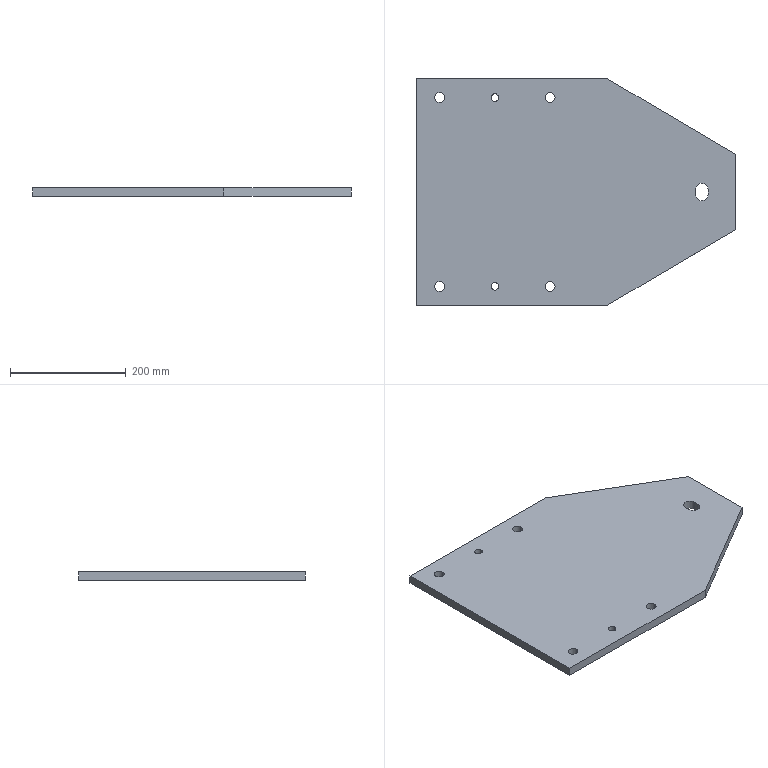Part | SolidWorks | features Extrusion 1, ICE 1 | 1 solid | 24 faces | box 550 x 390 x 15 mm | volume 2762557 mm3 | cylinder 14 | plane 10 | commonest cylinder face diameters 17 x8 13 x4 22 x2
STEP:
#1=CARTESIAN_POINT('',(-146.5,163.,0.));
#2=VERTEX_POINT('',#1);
#3=CARTESIAN_POINT('',(-133.5,163.,0.));
#4=VERTEX_POINT('',#3);
#5=CARTESIAN_POINT('',(-140.,163.,0.));
#6=DIRECTION('',(0.,0.,1.));
#7=DIRECTION('',(1.,0.,0.));
#8=AXIS2_PLACEMENT_3D('',#5,#6,#7);
#9=CIRCLE('',#8,6.5);
#10=EDGE_CURVE('',#2,#4,#9,.T.);
#11=ORIENTED_EDGE('',*,*,#10,.F.);
#12=CARTESIAN_POINT('',(-146.5,163.,15.));
#13=VERTEX_POINT('',#12);
#14=CARTESIAN_POINT('',(-146.5,163.,0.));
#15=DIRECTION('',(0.,0.,1.));
#16=VECTOR('',#15,1000.);
#17=LINE('',#14,#16);
#18=EDGE_CURVE('',#2,#13,#17,.T.);
#19=ORIENTED_EDGE('',*,*,#18,.T.);
#20=CARTESIAN_POINT('',(-133.5,163.,15.));
#21=VERTEX_POINT('',#20);
#22=CARTESIAN_POINT('',(-140.,163.,15.));
#23=DIRECTION('',(0.,0.,1.));
#24=DIRECTION('',(1.,0.,0.));
#25=AXIS2_PLACEMENT_3D('',#22,#23,#24);
#26=CIRCLE('',#25,6.5);
#27=EDGE_CURVE('',#13,#21,#26,.T.);
#28=ORIENTED_EDGE('',*,*,#27,.T.);
#29=CARTESIAN_POINT('',(-133.5,163.,0.));
#30=DIRECTION('',(0.,0.,1.));
#31=VECTOR('',#30,1000.);
#32=LINE('',#29,#31);
#33=EDGE_CURVE('',#4,#21,#32,.T.);
#34=ORIENTED_EDGE('',*,*,#33,.F.);
#35=EDGE_LOOP('',(#11,#19,#28,#34));
#36=FACE_OUTER_BOUND('',#35,.T.);
#37=CARTESIAN_POINT('',(-140.,163.,0.));
#38=DIRECTION('',(0.,0.,1.));
#39=DIRECTION('',(1.,0.,0.));
#40=AXIS2_PLACEMENT_3D('',#37,#38,#39);
#41=CYLINDRICAL_SURFACE('',#40,6.5);
#42=ADVANCED_FACE('',(#36),#41,.F.);
#43=CARTESIAN_POINT('',(-53.2,-163.,0.));
#44=VERTEX_POINT('',#43);
#45=CARTESIAN_POINT('',(-36.2,-163.,0.));
#46=VERTEX_POINT('',#45);
#47=CARTESIAN_POINT('',(-44.7,-163.,0.));
#48=DIRECTION('',(0.,0.,1.));
#49=DIRECTION('',(1.,0.,0.));
#50=AXIS2_PLACEMENT_3D('',#47,#48,#49);
#51=CIRCLE('',#50,8.5);
#52=EDGE_CURVE('',#44,#46,#51,.T.);
#53=ORIENTED_EDGE('',*,*,#52,.F.);
#54=CARTESIAN_POINT('',(-53.2,-163.,15.));
#55=VERTEX_POINT('',#54);
#56=CARTESIAN_POINT('',(-53.2,-163.,0.));
#57=DIRECTION('',(0.,0.,1.));
#58=VECTOR('',#57,1000.);
#59=LINE('',#56,#58);
#60=EDGE_CURVE('',#44,#55,#59,.T.);
#61=ORIENTED_EDGE('',*,*,#60,.T.);
#62=CARTESIAN_POINT('',(-36.2,-163.,15.));
#63=VERTEX_POINT('',#62);
#64=CARTESIAN_POINT('',(-44.7,-163.,15.));
#65=DIRECTION('',(0.,0.,1.));
#66=DIRECTION('',(1.,0.,0.));
#67=AXIS2_PLACEMENT_3D('',#64,#65,#66);
#68=CIRCLE('',#67,8.5);
#69=EDGE_CURVE('',#55,#63,#68,.T.);
#70=ORIENTED_EDGE('',*,*,#69,.T.);
#71=CARTESIAN_POINT('',(-36.2,-163.,0.));
#72=DIRECTION('',(0.,0.,1.));
#73=VECTOR('',#72,1000.);
#74=LINE('',#71,#73);
#75=EDGE_CURVE('',#46,#63,#74,.T.);
#76=ORIENTED_EDGE('',*,*,#75,.F.);
#77=EDGE_LOOP('',(#53,#61,#70,#76));
#78=FACE_OUTER_BOUND('',#77,.T.);
#79=CARTESIAN_POINT('',(-44.7,-163.,0.));
#80=DIRECTION('',(0.,0.,1.));
#81=DIRECTION('',(1.,0.,0.));
#82=AXIS2_PLACEMENT_3D('',#79,#80,#81);
#83=CYLINDRICAL_SURFACE('',#82,8.5);
#84=ADVANCED_FACE('',(#78),#83,.F.);
#85=CARTESIAN_POINT('',(-146.5,-163.,0.));
#86=VERTEX_POINT('',#85);
#87=CARTESIAN_POINT('',(-133.5,-163.,0.));
#88=VERTEX_POINT('',#87);
#89=CARTESIAN_POINT('',(-140.,-163.,0.));
#90=DIRECTION('',(0.,0.,1.));
#91=DIRECTION('',(1.,0.,0.));
#92=AXIS2_PLACEMENT_3D('',#89,#90,#91);
#93=CIRCLE('',#92,6.5);
#94=EDGE_CURVE('',#86,#88,#93,.T.);
#95=ORIENTED_EDGE('',*,*,#94,.F.);
#96=CARTESIAN_POINT('',(-146.5,-163.,15.));
#97=VERTEX_POINT('',#96);
#98=CARTESIAN_POINT('',(-146.5,-163.,0.));
#99=DIRECTION('',(0.,0.,1.));
#100=VECTOR('',#99,1000.);
#101=LINE('',#98,#100);
#102=EDGE_CURVE('',#86,#97,#101,.T.);
#103=ORIENTED_EDGE('',*,*,#102,.T.);
#104=CARTESIAN_POINT('',(-133.5,-163.,15.));
#105=VERTEX_POINT('',#104);
#106=CARTESIAN_POINT('',(-140.,-163.,15.));
#107=DIRECTION('',(0.,0.,1.));
#108=DIRECTION('',(1.,0.,0.));
#109=AXIS2_PLACEMENT_3D('',#106,#107,#108);
#110=CIRCLE('',#109,6.5);
#111=EDGE_CURVE('',#97,#105,#110,.T.);
#112=ORIENTED_EDGE('',*,*,#111,.T.);
#113=CARTESIAN_POINT('',(-133.5,-163.,0.));
#114=DIRECTION('',(0.,0.,1.));
#115=VECTOR('',#114,1000.);
#116=LINE('',#113,#115);
#117=EDGE_CURVE('',#88,#105,#116,.T.);
#118=ORIENTED_EDGE('',*,*,#117,.F.);
#119=EDGE_LOOP('',(#95,#103,#112,#118));
#120=FACE_OUTER_BOUND('',#119,.T.);
#121=CARTESIAN_POINT('',(-140.,-163.,0.));
#122=DIRECTION('',(0.,0.,1.));
#123=DIRECTION('',(1.,0.,0.));
#124=AXIS2_PLACEMENT_3D('',#121,#122,#123);
#125=CYLINDRICAL_SURFACE('',#124,6.5);
#126=ADVANCED_FACE('',(#120),#125,.F.);
#127=CARTESIAN_POINT('',(-243.7,-163.,0.));
#128=VERTEX_POINT('',#127);
#129=CARTESIAN_POINT('',(-226.7,-163.,0.));
#130=VERTEX_POINT('',#129);
#131=CARTESIAN_POINT('',(-235.2,-163.,0.));
#132=DIRECTION('',(0.,0.,1.));
#133=DIRECTION('',(1.,0.,0.));
#134=AXIS2_PLACEMENT_3D('',#131,#132,#133);
#135=CIRCLE('',#134,8.5);
#136=EDGE_CURVE('',#128,#130,#135,.T.);
#137=ORIENTED_EDGE('',*,*,#136,.F.);
#138=CARTESIAN_POINT('',(-243.7,-163.,15.));
#139=VERTEX_POINT('',#138);
#140=CARTESIAN_POINT('',(-243.7,-163.,0.));
#141=DIRECTION('',(0.,0.,1.));
#142=VECTOR('',#141,1000.);
#143=LINE('',#140,#142);
#144=EDGE_CURVE('',#128,#139,#143,.T.);
#145=ORIENTED_EDGE('',*,*,#144,.T.);
#146=CARTESIAN_POINT('',(-226.7,-163.,15.));
#147=VERTEX_POINT('',#146);
#148=CARTESIAN_POINT('',(-235.2,-163.,15.));
#149=DIRECTION('',(0.,0.,1.));
#150=DIRECTION('',(1.,0.,0.));
#151=AXIS2_PLACEMENT_3D('',#148,#149,#150);
#152=CIRCLE('',#151,8.5);
#153=EDGE_CURVE('',#139,#147,#152,.T.);
#154=ORIENTED_EDGE('',*,*,#153,.T.);
#155=CARTESIAN_POINT('',(-226.7,-163.,0.));
#156=DIRECTION('',(0.,0.,1.));
#157=VECTOR('',#156,1000.);
#158=LINE('',#155,#157);
#159=EDGE_CURVE('',#130,#147,#158,.T.);
#160=ORIENTED_EDGE('',*,*,#159,.F.);
#161=EDGE_LOOP('',(#137,#145,#154,#160));
#162=FACE_OUTER_BOUND('',#161,.T.);
#163=CARTESIAN_POINT('',(-235.2,-163.,0.));
#164=DIRECTION('',(0.,0.,1.));
#165=DIRECTION('',(1.,0.,0.));
#166=AXIS2_PLACEMENT_3D('',#163,#164,#165);
#167=CYLINDRICAL_SURFACE('',#166,8.5);
#168=ADVANCED_FACE('',(#162),#167,.F.);
#169=CARTESIAN_POINT('',(-53.2,163.,0.));
#170=VERTEX_POINT('',#169);
#171=CARTESIAN_POINT('',(-36.2,163.,0.));
#172=VERTEX_POINT('',#171);
#173=CARTESIAN_POINT('',(-44.7,163.,0.));
#174=DIRECTION('',(0.,0.,1.));
#175=DIRECTION('',(1.,0.,0.));
#176=AXIS2_PLACEMENT_3D('',#173,#174,#175);
#177=CIRCLE('',#176,8.5);
#178=EDGE_CURVE('',#170,#172,#177,.T.);
#179=ORIENTED_EDGE('',*,*,#178,.F.);
#180=CARTESIAN_POINT('',(-53.2,163.,15.));
#181=VERTEX_POINT('',#180);
#182=CARTESIAN_POINT('',(-53.2,163.,0.));
#183=DIRECTION('',(0.,0.,1.));
#184=VECTOR('',#183,1000.);
#185=LINE('',#182,#184);
#186=EDGE_CURVE('',#170,#181,#185,.T.);
#187=ORIENTED_EDGE('',*,*,#186,.T.);
#188=CARTESIAN_POINT('',(-36.2,163.,15.));
#189=VERTEX_POINT('',#188);
#190=CARTESIAN_POINT('',(-44.7,163.,15.));
#191=DIRECTION('',(0.,0.,1.));
#192=DIRECTION('',(1.,0.,0.));
#193=AXIS2_PLACEMENT_3D('',#190,#191,#192);
#194=CIRCLE('',#193,8.5);
#195=EDGE_CURVE('',#181,#189,#194,.T.);
#196=ORIENTED_EDGE('',*,*,#195,.T.);
#197=CARTESIAN_POINT('',(-36.2,163.,0.));
#198=DIRECTION('',(0.,0.,1.));
#199=VECTOR('',#198,1000.);
#200=LINE('',#197,#199);
#201=EDGE_CURVE('',#172,#189,#200,.T.);
#202=ORIENTED_EDGE('',*,*,#201,.F.);
#203=EDGE_LOOP('',(#179,#187,#196,#202));
#204=FACE_OUTER_BOUND('',#203,.T.);
#205=CARTESIAN_POINT('',(-44.7,163.,0.));
#206=DIRECTION('',(0.,0.,1.));
#207=DIRECTION('',(1.,0.,0.));
#208=AXIS2_PLACEMENT_3D('',#205,#206,#207);
#209=CYLINDRICAL_SURFACE('',#208,8.5);
#210=ADVANCED_FACE('',(#204),#209,.F.);
#211=CARTESIAN_POINT('',(-243.7,163.,0.));
#212=VERTEX_POINT('',#211);
#213=CARTESIAN_POINT('',(-226.7,163.,0.));
#214=VERTEX_POINT('',#213);
#215=CARTESIAN_POINT('',(-235.2,163.,0.));
#216=DIRECTION('',(0.,0.,1.));
#217=DIRECTION('',(1.,0.,0.));
#218=AXIS2_PLACEMENT_3D('',#215,#216,#217);
#219=CIRCLE('',#218,8.5);
#220=EDGE_CURVE('',#212,#214,#219,.T.);
#221=ORIENTED_EDGE('',*,*,#220,.F.);
#222=CARTESIAN_POINT('',(-243.7,163.,15.));
#223=VERTEX_POINT('',#222);
#224=CARTESIAN_POINT('',(-243.7,163.,0.));
#225=DIRECTION('',(0.,0.,1.));
#226=VECTOR('',#225,1000.);
#227=LINE('',#224,#226);
#228=EDGE_CURVE('',#212,#223,#227,.T.);
#229=ORIENTED_EDGE('',*,*,#228,.T.);
#230=CARTESIAN_POINT('',(-226.7,163.,15.));
#231=VERTEX_POINT('',#230);
#232=CARTESIAN_POINT('',(-235.2,163.,15.));
#233=DIRECTION('',(0.,0.,1.));
#234=DIRECTION('',(1.,0.,0.));
#235=AXIS2_PLACEMENT_3D('',#232,#233,#234);
#236=CIRCLE('',#235,8.5);
#237=EDGE_CURVE('',#223,#231,#236,.T.);
#238=ORIENTED_EDGE('',*,*,#237,.T.);
#239=CARTESIAN_POINT('',(-226.7,163.,0.));
#240=DIRECTION('',(0.,0.,1.));
#241=VECTOR('',#240,1000.);
#242=LINE('',#239,#241);
#243=EDGE_CURVE('',#214,#231,#242,.T.);
#244=ORIENTED_EDGE('',*,*,#243,.F.);
#245=EDGE_LOOP('',(#221,#229,#238,#244));
#246=FACE_OUTER_BOUND('',#245,.T.);
#247=CARTESIAN_POINT('',(-235.2,163.,0.));
#248=DIRECTION('',(0.,0.,1.));
#249=DIRECTION('',(1.,0.,0.));
#250=AXIS2_PLACEMENT_3D('',#247,#248,#249);
#251=CYLINDRICAL_SURFACE('',#250,8.5);
#252=ADVANCED_FACE('',(#246),#251,.F.);
#253=CARTESIAN_POINT('',(-275.,195.,0.));
#254=VERTEX_POINT('',#253);
#255=CARTESIAN_POINT('',(-275.,-195.,0.));
#256=VERTEX_POINT('',#255);
#257=CARTESIAN_POINT('',(-275.,195.,0.));
#258=DIRECTION('',(0.,-1.,0.));
#259=VECTOR('',#258,1000.);
#260=LINE('',#257,#259);
#261=EDGE_CURVE('',#254,#256,#260,.T.);
#262=ORIENTED_EDGE('',*,*,#261,.T.);
#263=CARTESIAN_POINT('',(-275.,-195.,15.));
#264=VERTEX_POINT('',#263);
#265=CARTESIAN_POINT('',(-275.,-195.,15.));
#266=DIRECTION('',(0.,0.,-1.));
#267=VECTOR('',#266,1000.);
#268=LINE('',#265,#267);
#269=EDGE_CURVE('',#264,#256,#268,.T.);
#270=ORIENTED_EDGE('',*,*,#269,.F.);
#271=CARTESIAN_POINT('',(-275.,195.,15.));
#272=VERTEX_POINT('',#271);
#273=CARTESIAN_POINT('',(-275.,195.,15.));
#274=DIRECTION('',(0.,-1.,0.));
#275=VECTOR('',#274,1000.);
#276=LINE('',#273,#275);
#277=EDGE_CURVE('',#272,#264,#276,.T.);
#278=ORIENTED_EDGE('',*,*,#277,.F.);
#279=CARTESIAN_POINT('',(-275.,195.,15.));
#280=DIRECTION('',(0.,0.,-1.));
#281=VECTOR('',#280,1000.);
#282=LINE('',#279,#281);
#283=EDGE_CURVE('',#272,#254,#282,.T.);
#284=ORIENTED_EDGE('',*,*,#283,.T.);
#285=EDGE_LOOP('',(#262,#270,#278,#284));
#286=FACE_OUTER_BOUND('',#285,.T.);
#287=CARTESIAN_POINT('',(-275.,195.,15.));
#288=DIRECTION('',(1.,0.,0.));
#289=DIRECTION('',(0.,1.,0.));
#290=AXIS2_PLACEMENT_3D('',#287,#288,#289);
#291=PLANE('',#290);
#292=ADVANCED_FACE('',(#286),#291,.F.);
#293=CARTESIAN_POINT('',(55.,-195.,0.));
#294=VERTEX_POINT('',#293);
#295=CARTESIAN_POINT('',(275.,-195.,0.));
#296=DIRECTION('',(1.,0.,0.));
#297=VECTOR('',#296,1000.);
#298=LINE('',#295,#297);
#299=EDGE_CURVE('',#256,#294,#298,.T.);
#300=ORIENTED_EDGE('',*,*,#299,.T.);
#301=CARTESIAN_POINT('',(55.,-195.,15.));
#302=VERTEX_POINT('',#301);
#303=CARTESIAN_POINT('',(55.,-195.,0.));
#304=DIRECTION('',(0.,0.,1.));
#305=VECTOR('',#304,1000.);
#306=LINE('',#303,#305);
#307=EDGE_CURVE('',#294,#302,#306,.T.);
#308=ORIENTED_EDGE('',*,*,#307,.T.);
#309=CARTESIAN_POINT('',(275.,-195.,15.));
#310=DIRECTION('',(1.,0.,0.));
#311=VECTOR('',#310,1000.);
#312=LINE('',#309,#311);
#313=EDGE_CURVE('',#264,#302,#312,.T.);
#314=ORIENTED_EDGE('',*,*,#313,.F.);
#315=ORIENTED_EDGE('',*,*,#269,.T.);
#316=EDGE_LOOP('',(#300,#308,#314,#315));
#317=FACE_OUTER_BOUND('',#316,.T.);
#318=CARTESIAN_POINT('',(275.,-195.,15.));
#319=DIRECTION('',(0.,1.,0.));
#320=DIRECTION('',(-1.,0.,0.));
#321=AXIS2_PLACEMENT_3D('',#318,#319,#320);
#322=PLANE('',#321);
#323=ADVANCED_FACE('',(#317),#322,.F.);
#324=CARTESIAN_POINT('',(275.,-65.,0.));
#325=VERTEX_POINT('',#324);
#326=CARTESIAN_POINT('',(275.,65.,0.));
#327=VERTEX_POINT('',#326);
#328=CARTESIAN_POINT('',(275.,195.,0.));
#329=DIRECTION('',(0.,1.,0.));
#330=VECTOR('',#329,1000.);
#331=LINE('',#328,#330);
#332=EDGE_CURVE('',#325,#327,#331,.T.);
#333=ORIENTED_EDGE('',*,*,#332,.T.);
#334=CARTESIAN_POINT('',(275.,65.,15.));
#335=VERTEX_POINT('',#334);
#336=CARTESIAN_POINT('',(275.,65.,0.));
#337=DIRECTION('',(0.,0.,1.));
#338=VECTOR('',#337,1000.);
#339=LINE('',#336,#338);
#340=EDGE_CURVE('',#327,#335,#339,.T.);
#341=ORIENTED_EDGE('',*,*,#340,.T.);
#342=CARTESIAN_POINT('',(275.,-65.,15.));
#343=VERTEX_POINT('',#342);
#344=CARTESIAN_POINT('',(275.,195.,15.));
#345=DIRECTION('',(0.,1.,0.));
#346=VECTOR('',#345,1000.);
#347=LINE('',#344,#346);
#348=EDGE_CURVE('',#343,#335,#347,.T.);
#349=ORIENTED_EDGE('',*,*,#348,.F.);
#350=CARTESIAN_POINT('',(275.,-65.,0.));
#351=DIRECTION('',(0.,0.,1.));
#352=VECTOR('',#351,1000.);
#353=LINE('',#350,#352);
#354=EDGE_CURVE('',#325,#343,#353,.T.);
#355=ORIENTED_EDGE('',*,*,#354,.F.);
#356=EDGE_LOOP('',(#333,#341,#349,#355));
#357=FACE_OUTER_BOUND('',#356,.T.);
#358=CARTESIAN_POINT('',(275.,195.,15.));
#359=DIRECTION('',(-1.,0.,0.));
#360=DIRECTION('',(0.,-1.,0.));
#361=AXIS2_PLACEMENT_3D('',#358,#359,#360);
#362=PLANE('',#361);
#363=ADVANCED_FACE('',(#357),#362,.F.);
#364=CARTESIAN_POINT('',(55.,195.,15.));
#365=VERTEX_POINT('',#364);
#366=CARTESIAN_POINT('',(275.,195.,15.));
#367=DIRECTION('',(-1.,0.,0.));
#368=VECTOR('',#367,1000.);
#369=LINE('',#366,#368);
#370=EDGE_CURVE('',#365,#272,#369,.T.);
#371=ORIENTED_EDGE('',*,*,#370,.F.);
#372=CARTESIAN_POINT('',(55.,195.,0.));
#373=VERTEX_POINT('',#372);
#374=CARTESIAN_POINT('',(55.,195.,0.));
#375=DIRECTION('',(0.,0.,1.));
#376=VECTOR('',#375,1000.);
#377=LINE('',#374,#376);
#378=EDGE_CURVE('',#373,#365,#377,.T.);
#379=ORIENTED_EDGE('',*,*,#378,.F.);
#380=CARTESIAN_POINT('',(275.,195.,0.));
#381=DIRECTION('',(-1.,0.,0.));
#382=VECTOR('',#381,1000.);
#383=LINE('',#380,#382);
#384=EDGE_CURVE('',#373,#254,#383,.T.);
#385=ORIENTED_EDGE('',*,*,#384,.T.);
#386=ORIENTED_EDGE('',*,*,#283,.F.);
#387=EDGE_LOOP('',(#371,#379,#385,#386));
#388=FACE_OUTER_BOUND('',#387,.T.);
#389=CARTESIAN_POINT('',(275.,195.,15.));
#390=DIRECTION('',(0.,-1.,0.));
#391=DIRECTION('',(1.,0.,0.));
#392=AXIS2_PLACEMENT_3D('',#389,#390,#391);
#393=PLANE('',#392);
#394=ADVANCED_FACE('',(#388),#393,.F.);
#395=CARTESIAN_POINT('',(-140.,163.,15.));
#396=DIRECTION('',(0.,0.,1.));
#397=DIRECTION('',(1.,0.,0.));
#398=AXIS2_PLACEMENT_3D('',#395,#396,#397);
#399=CIRCLE('',#398,6.5);
#400=EDGE_CURVE('',#21,#13,#399,.T.);
#401=ORIENTED_EDGE('',*,*,#400,.F.);
#402=ORIENTED_EDGE('',*,*,#27,.F.);
#403=EDGE_LOOP('',(#401,#402));
#404=FACE_BOUND('',#403,.T.);
#405=CARTESIAN_POINT('',(-44.7,-163.,15.));
#406=DIRECTION('',(0.,0.,1.));
#407=DIRECTION('',(1.,0.,0.));
#408=AXIS2_PLACEMENT_3D('',#405,#406,#407);
#409=CIRCLE('',#408,8.5);
#410=EDGE_CURVE('',#63,#55,#409,.T.);
#411=ORIENTED_EDGE('',*,*,#410,.F.);
#412=ORIENTED_EDGE('',*,*,#69,.F.);
#413=EDGE_LOOP('',(#411,#412));
#414=FACE_BOUND('',#413,.T.);
#415=CARTESIAN_POINT('',(-140.,-163.,15.));
#416=DIRECTION('',(0.,0.,1.));
#417=DIRECTION('',(1.,0.,0.));
#418=AXIS2_PLACEMENT_3D('',#415,#416,#417);
#419=CIRCLE('',#418,6.5);
#420=EDGE_CURVE('',#105,#97,#419,.T.);
#421=ORIENTED_EDGE('',*,*,#420,.F.);
#422=ORIENTED_EDGE('',*,*,#111,.F.);
#423=EDGE_LOOP('',(#421,#422));
#424=FACE_BOUND('',#423,.T.);
#425=CARTESIAN_POINT('',(-235.2,-163.,15.));
#426=DIRECTION('',(0.,0.,1.));
#427=DIRECTION('',(1.,0.,0.));
#428=AXIS2_PLACEMENT_3D('',#425,#426,#427);
#429=CIRCLE('',#428,8.5);
#430=EDGE_CURVE('',#147,#139,#429,.T.);
#431=ORIENTED_EDGE('',*,*,#430,.F.);
#432=ORIENTED_EDGE('',*,*,#153,.F.);
#433=EDGE_LOOP('',(#431,#432));
#434=FACE_BOUND('',#433,.T.);
#435=CARTESIAN_POINT('',(206.,4.,15.));
#436=VERTEX_POINT('',#435);
#437=CARTESIAN_POINT('',(206.,-4.,15.));
#438=VERTEX_POINT('',#437);
#439=CARTESIAN_POINT('',(206.,4.,15.));
#440=DIRECTION('',(0.,-1.,0.));
#441=VECTOR('',#440,1000.);
#442=LINE('',#439,#441);
#443=EDGE_CURVE('',#436,#438,#442,.T.);
#444=ORIENTED_EDGE('',*,*,#443,.F.);
#445=CARTESIAN_POINT('',(228.,4.,15.));
#446=VERTEX_POINT('',#445);
#447=CARTESIAN_POINT('',(217.,4.,15.));
#448=DIRECTION('',(0.,0.,1.));
#449=DIRECTION('',(1.,0.,0.));
#450=AXIS2_PLACEMENT_3D('',#447,#448,#449);
#451=CIRCLE('',#450,11.);
#452=EDGE_CURVE('',#446,#436,#451,.T.);
#453=ORIENTED_EDGE('',*,*,#452,.F.);
#454=CARTESIAN_POINT('',(228.,-4.,15.));
#455=VERTEX_POINT('',#454);
#456=CARTESIAN_POINT('',(228.,4.,15.));
#457=DIRECTION('',(0.,1.,0.));
#458=VECTOR('',#457,1000.);
#459=LINE('',#456,#458);
#460=EDGE_CURVE('',#455,#446,#459,.T.);
#461=ORIENTED_EDGE('',*,*,#460,.F.);
#462=CARTESIAN_POINT('',(217.,-4.,15.));
#463=DIRECTION('',(0.,0.,1.));
#464=DIRECTION('',(1.,0.,0.));
#465=AXIS2_PLACEMENT_3D('',#462,#463,#464);
#466=CIRCLE('',#465,11.);
#467=EDGE_CURVE('',#438,#455,#466,.T.);
#468=ORIENTED_EDGE('',*,*,#467,.F.);
#469=EDGE_LOOP('',(#444,#453,#461,#468));
#470=FACE_BOUND('',#469,.T.);
#471=CARTESIAN_POINT('',(-44.7,163.,15.));
#472=DIRECTION('',(0.,0.,1.));
#473=DIRECTION('',(1.,0.,0.));
#474=AXIS2_PLACEMENT_3D('',#471,#472,#473);
#475=CIRCLE('',#474,8.5);
#476=EDGE_CURVE('',#189,#181,#475,.T.);
#477=ORIENTED_EDGE('',*,*,#476,.F.);
#478=ORIENTED_EDGE('',*,*,#195,.F.);
#479=EDGE_LOOP('',(#477,#478));
#480=FACE_BOUND('',#479,.T.);
#481=CARTESIAN_POINT('',(-235.2,163.,15.));
#482=DIRECTION('',(0.,0.,1.));
#483=DIRECTION('',(1.,0.,0.));
#484=AXIS2_PLACEMENT_3D('',#481,#482,#483);
#485=CIRCLE('',#484,8.5);
#486=EDGE_CURVE('',#231,#223,#485,.T.);
#487=ORIENTED_EDGE('',*,*,#486,.F.);
#488=ORIENTED_EDGE('',*,*,#237,.F.);
#489=EDGE_LOOP('',(#487,#488));
#490=FACE_BOUND('',#489,.T.);
#491=ORIENTED_EDGE('',*,*,#348,.T.);
#492=CARTESIAN_POINT('',(55.,195.,15.));
#493=DIRECTION('',(0.8609,-0.5087,0.));
#494=VECTOR('',#493,1000.);
#495=LINE('',#492,#494);
#496=EDGE_CURVE('',#365,#335,#495,.T.);
#497=ORIENTED_EDGE('',*,*,#496,.F.);
#498=ORIENTED_EDGE('',*,*,#370,.T.);
#499=ORIENTED_EDGE('',*,*,#277,.T.);
#500=ORIENTED_EDGE('',*,*,#313,.T.);
#501=CARTESIAN_POINT('',(55.,-195.,15.));
#502=DIRECTION('',(-0.8609,-0.5087,0.));
#503=VECTOR('',#502,1000.);
#504=LINE('',#501,#503);
#505=EDGE_CURVE('',#343,#302,#504,.T.);
#506=ORIENTED_EDGE('',*,*,#505,.F.);
#507=EDGE_LOOP('',(#491,#497,#498,#499,#500,#506));
#508=FACE_OUTER_BOUND('',#507,.T.);
#509=CARTESIAN_POINT('',(0.,0.,15.));
#510=DIRECTION('',(0.,0.,-1.));
#511=DIRECTION('',(-1.,0.,0.));
#512=AXIS2_PLACEMENT_3D('',#509,#510,#511);
#513=PLANE('',#512);
#514=ADVANCED_FACE('',(#404,#414,#424,#434,#470,#480,#490,#508),#513,.F.);
#515=CARTESIAN_POINT('',(-140.,163.,0.));
#516=DIRECTION('',(0.,0.,1.));
#517=DIRECTION('',(1.,0.,0.));
#518=AXIS2_PLACEMENT_3D('',#515,#516,#517);
#519=CIRCLE('',#518,6.5);
#520=EDGE_CURVE('',#4,#2,#519,.T.);
#521=ORIENTED_EDGE('',*,*,#520,.T.);
#522=ORIENTED_EDGE('',*,*,#10,.T.);
#523=EDGE_LOOP('',(#521,#522));
#524=FACE_BOUND('',#523,.T.);
#525=CARTESIAN_POINT('',(-44.7,-163.,0.));
#526=DIRECTION('',(0.,0.,1.));
#527=DIRECTION('',(1.,0.,0.));
#528=AXIS2_PLACEMENT_3D('',#525,#526,#527);
#529=CIRCLE('',#528,8.5);
#530=EDGE_CURVE('',#46,#44,#529,.T.);
#531=ORIENTED_EDGE('',*,*,#530,.T.);
#532=ORIENTED_EDGE('',*,*,#52,.T.);
#533=EDGE_LOOP('',(#531,#532));
#534=FACE_BOUND('',#533,.T.);
#535=CARTESIAN_POINT('',(-140.,-163.,0.));
#536=DIRECTION('',(0.,0.,1.));
#537=DIRECTION('',(1.,0.,0.));
#538=AXIS2_PLACEMENT_3D('',#535,#536,#537);
#539=CIRCLE('',#538,6.5);
#540=EDGE_CURVE('',#88,#86,#539,.T.);
#541=ORIENTED_EDGE('',*,*,#540,.T.);
#542=ORIENTED_EDGE('',*,*,#94,.T.);
#543=EDGE_LOOP('',(#541,#542));
#544=FACE_BOUND('',#543,.T.);
#545=CARTESIAN_POINT('',(-235.2,-163.,0.));
#546=DIRECTION('',(0.,0.,1.));
#547=DIRECTION('',(1.,0.,0.));
#548=AXIS2_PLACEMENT_3D('',#545,#546,#547);
#549=CIRCLE('',#548,8.5);
#550=EDGE_CURVE('',#130,#128,#549,.T.);
#551=ORIENTED_EDGE('',*,*,#550,.T.);
#552=ORIENTED_EDGE('',*,*,#136,.T.);
#553=EDGE_LOOP('',(#551,#552));
#554=FACE_BOUND('',#553,.T.);
#555=CARTESIAN_POINT('',(228.,4.,0.));
#556=VERTEX_POINT('',#555);
#557=CARTESIAN_POINT('',(206.,4.,0.));
#558=VERTEX_POINT('',#557);
#559=CARTESIAN_POINT('',(217.,4.,0.));
#560=DIRECTION('',(0.,0.,1.));
#561=DIRECTION('',(1.,0.,0.));
#562=AXIS2_PLACEMENT_3D('',#559,#560,#561);
#563=CIRCLE('',#562,11.);
#564=EDGE_CURVE('',#556,#558,#563,.T.);
#565=ORIENTED_EDGE('',*,*,#564,.T.);
#566=CARTESIAN_POINT('',(206.,-4.,0.));
#567=VERTEX_POINT('',#566);
#568=CARTESIAN_POINT('',(206.,4.,0.));
#569=DIRECTION('',(0.,-1.,0.));
#570=VECTOR('',#569,1000.);
#571=LINE('',#568,#570);
#572=EDGE_CURVE('',#558,#567,#571,.T.);
#573=ORIENTED_EDGE('',*,*,#572,.T.);
#574=CARTESIAN_POINT('',(228.,-4.,0.));
#575=VERTEX_POINT('',#574);
#576=CARTESIAN_POINT('',(217.,-4.,0.));
#577=DIRECTION('',(0.,0.,1.));
#578=DIRECTION('',(1.,0.,0.));
#579=AXIS2_PLACEMENT_3D('',#576,#577,#578);
#580=CIRCLE('',#579,11.);
#581=EDGE_CURVE('',#567,#575,#580,.T.);
#582=ORIENTED_EDGE('',*,*,#581,.T.);
#583=CARTESIAN_POINT('',(228.,4.,0.));
#584=DIRECTION('',(0.,1.,0.));
#585=VECTOR('',#584,1000.);
#586=LINE('',#583,#585);
#587=EDGE_CURVE('',#575,#556,#586,.T.);
#588=ORIENTED_EDGE('',*,*,#587,.T.);
#589=EDGE_LOOP('',(#565,#573,#582,#588));
#590=FACE_BOUND('',#589,.T.);
#591=CARTESIAN_POINT('',(55.,195.,0.));
#592=DIRECTION('',(0.8609,-0.5087,0.));
#593=VECTOR('',#592,1000.);
#594=LINE('',#591,#593);
#595=EDGE_CURVE('',#373,#327,#594,.T.);
#596=ORIENTED_EDGE('',*,*,#595,.T.);
#597=ORIENTED_EDGE('',*,*,#332,.F.);
#598=CARTESIAN_POINT('',(55.,-195.,0.));
#599=DIRECTION('',(-0.8609,-0.5087,0.));
#600=VECTOR('',#599,1000.);
#601=LINE('',#598,#600);
#602=EDGE_CURVE('',#325,#294,#601,.T.);
#603=ORIENTED_EDGE('',*,*,#602,.T.);
#604=ORIENTED_EDGE('',*,*,#299,.F.);
#605=ORIENTED_EDGE('',*,*,#261,.F.);
#606=ORIENTED_EDGE('',*,*,#384,.F.);
#607=EDGE_LOOP('',(#596,#597,#603,#604,#605,#606));
#608=FACE_OUTER_BOUND('',#607,.T.);
#609=CARTESIAN_POINT('',(-44.7,163.,0.));
#610=DIRECTION('',(0.,0.,1.));
#611=DIRECTION('',(1.,0.,0.));
#612=AXIS2_PLACEMENT_3D('',#609,#610,#611);
#613=CIRCLE('',#612,8.5);
#614=EDGE_CURVE('',#172,#170,#613,.T.);
#615=ORIENTED_EDGE('',*,*,#614,.T.);
#616=ORIENTED_EDGE('',*,*,#178,.T.);
#617=EDGE_LOOP('',(#615,#616));
#618=FACE_BOUND('',#617,.T.);
#619=CARTESIAN_POINT('',(-235.2,163.,0.));
#620=DIRECTION('',(0.,0.,1.));
#621=DIRECTION('',(1.,0.,0.));
#622=AXIS2_PLACEMENT_3D('',#619,#620,#621);
#623=CIRCLE('',#622,8.5);
#624=EDGE_CURVE('',#214,#212,#623,.T.);
#625=ORIENTED_EDGE('',*,*,#624,.T.);
#626=ORIENTED_EDGE('',*,*,#220,.T.);
#627=EDGE_LOOP('',(#625,#626));
#628=FACE_BOUND('',#627,.T.);
#629=CARTESIAN_POINT('',(0.,0.,0.));
#630=DIRECTION('',(0.,0.,-1.));
#631=DIRECTION('',(-1.,0.,0.));
#632=AXIS2_PLACEMENT_3D('',#629,#630,#631);
#633=PLANE('',#632);
#634=ADVANCED_FACE('',(#524,#534,#544,#554,#590,#608,#618,#628),#633,.T.);
#635=ORIENTED_EDGE('',*,*,#228,.F.);
#636=ORIENTED_EDGE('',*,*,#624,.F.);
#637=ORIENTED_EDGE('',*,*,#243,.T.);
#638=ORIENTED_EDGE('',*,*,#486,.T.);
#639=EDGE_LOOP('',(#635,#636,#637,#638));
#640=FACE_OUTER_BOUND('',#639,.T.);
#641=CARTESIAN_POINT('',(-235.2,163.,0.));
#642=DIRECTION('',(0.,0.,1.));
#643=DIRECTION('',(1.,0.,0.));
#644=AXIS2_PLACEMENT_3D('',#641,#642,#643);
#645=CYLINDRICAL_SURFACE('',#644,8.5);
#646=ADVANCED_FACE('',(#640),#645,.F.);
#647=ORIENTED_EDGE('',*,*,#186,.F.);
#648=ORIENTED_EDGE('',*,*,#614,.F.);
#649=ORIENTED_EDGE('',*,*,#201,.T.);
#650=ORIENTED_EDGE('',*,*,#476,.T.);
#651=EDGE_LOOP('',(#647,#648,#649,#650));
#652=FACE_OUTER_BOUND('',#651,.T.);
#653=CARTESIAN_POINT('',(-44.7,163.,0.));
#654=DIRECTION('',(0.,0.,1.));
#655=DIRECTION('',(1.,0.,0.));
#656=AXIS2_PLACEMENT_3D('',#653,#654,#655);
#657=CYLINDRICAL_SURFACE('',#656,8.5);
#658=ADVANCED_FACE('',(#652),#657,.F.);
#659=ORIENTED_EDGE('',*,*,#505,.T.);
#660=ORIENTED_EDGE('',*,*,#307,.F.);
#661=ORIENTED_EDGE('',*,*,#602,.F.);
#662=ORIENTED_EDGE('',*,*,#354,.T.);
#663=EDGE_LOOP('',(#659,#660,#661,#662));
#664=FACE_OUTER_BOUND('',#663,.T.);
#665=CARTESIAN_POINT('',(55.,-195.,0.));
#666=DIRECTION('',(-0.5087,0.8609,0.));
#667=DIRECTION('',(-0.8609,-0.5087,0.));
#668=AXIS2_PLACEMENT_3D('',#665,#666,#667);
#669=PLANE('',#668);
#670=ADVANCED_FACE('',(#664),#669,.F.);
#671=ORIENTED_EDGE('',*,*,#496,.T.);
#672=ORIENTED_EDGE('',*,*,#340,.F.);
#673=ORIENTED_EDGE('',*,*,#595,.F.);
#674=ORIENTED_EDGE('',*,*,#378,.T.);
#675=EDGE_LOOP('',(#671,#672,#673,#674));
#676=FACE_OUTER_BOUND('',#675,.T.);
#677=CARTESIAN_POINT('',(55.,195.,0.));
#678=DIRECTION('',(-0.5087,-0.8609,0.));
#679=DIRECTION('',(0.8609,-0.5087,0.));
#680=AXIS2_PLACEMENT_3D('',#677,#678,#679);
#681=PLANE('',#680);
#682=ADVANCED_FACE('',(#676),#681,.F.);
#683=ORIENTED_EDGE('',*,*,#452,.T.);
#684=CARTESIAN_POINT('',(206.,4.,0.));
#685=DIRECTION('',(0.,0.,1.));
#686=VECTOR('',#685,1000.);
#687=LINE('',#684,#686);
#688=EDGE_CURVE('',#558,#436,#687,.T.);
#689=ORIENTED_EDGE('',*,*,#688,.F.);
#690=ORIENTED_EDGE('',*,*,#564,.F.);
#691=CARTESIAN_POINT('',(228.,4.,0.));
#692=DIRECTION('',(0.,0.,1.));
#693=VECTOR('',#692,1000.);
#694=LINE('',#691,#693);
#695=EDGE_CURVE('',#556,#446,#694,.T.);
#696=ORIENTED_EDGE('',*,*,#695,.T.);
#697=EDGE_LOOP('',(#683,#689,#690,#696));
#698=FACE_OUTER_BOUND('',#697,.T.);
#699=CARTESIAN_POINT('',(217.,4.,0.));
#700=DIRECTION('',(0.,0.,1.));
#701=DIRECTION('',(1.,0.,0.));
#702=AXIS2_PLACEMENT_3D('',#699,#700,#701);
#703=CYLINDRICAL_SURFACE('',#702,11.);
#704=ADVANCED_FACE('',(#698),#703,.F.);
#705=ORIENTED_EDGE('',*,*,#460,.T.);
#706=ORIENTED_EDGE('',*,*,#695,.F.);
#707=ORIENTED_EDGE('',*,*,#587,.F.);
#708=CARTESIAN_POINT('',(228.,-4.,0.));
#709=DIRECTION('',(0.,0.,1.));
#710=VECTOR('',#709,1000.);
#711=LINE('',#708,#710);
#712=EDGE_CURVE('',#575,#455,#711,.T.);
#713=ORIENTED_EDGE('',*,*,#712,.T.);
#714=EDGE_LOOP('',(#705,#706,#707,#713));
#715=FACE_OUTER_BOUND('',#714,.T.);
#716=CARTESIAN_POINT('',(228.,4.,0.));
#717=DIRECTION('',(1.,0.,0.));
#718=DIRECTION('',(0.,0.,-1.));
#719=AXIS2_PLACEMENT_3D('',#716,#717,#718);
#720=PLANE('',#719);
#721=ADVANCED_FACE('',(#715),#720,.F.);
#722=ORIENTED_EDGE('',*,*,#467,.T.);
#723=ORIENTED_EDGE('',*,*,#712,.F.);
#724=ORIENTED_EDGE('',*,*,#581,.F.);
#725=CARTESIAN_POINT('',(206.,-4.,0.));
#726=DIRECTION('',(0.,0.,1.));
#727=VECTOR('',#726,1000.);
#728=LINE('',#725,#727);
#729=EDGE_CURVE('',#567,#438,#728,.T.);
#730=ORIENTED_EDGE('',*,*,#729,.T.);
#731=EDGE_LOOP('',(#722,#723,#724,#730));
#732=FACE_OUTER_BOUND('',#731,.T.);
#733=CARTESIAN_POINT('',(217.,-4.,0.));
#734=DIRECTION('',(0.,0.,1.));
#735=DIRECTION('',(1.,0.,0.));
#736=AXIS2_PLACEMENT_3D('',#733,#734,#735);
#737=CYLINDRICAL_SURFACE('',#736,11.);
#738=ADVANCED_FACE('',(#732),#737,.F.);
#739=ORIENTED_EDGE('',*,*,#443,.T.);
#740=ORIENTED_EDGE('',*,*,#729,.F.);
#741=ORIENTED_EDGE('',*,*,#572,.F.);
#742=ORIENTED_EDGE('',*,*,#688,.T.);
#743=EDGE_LOOP('',(#739,#740,#741,#742));
#744=FACE_OUTER_BOUND('',#743,.T.);
#745=CARTESIAN_POINT('',(206.,4.,0.));
#746=DIRECTION('',(-1.,0.,0.));
#747=DIRECTION('',(0.,0.,1.));
#748=AXIS2_PLACEMENT_3D('',#745,#746,#747);
#749=PLANE('',#748);
#750=ADVANCED_FACE('',(#744),#749,.F.);
#751=ORIENTED_EDGE('',*,*,#144,.F.);
#752=ORIENTED_EDGE('',*,*,#550,.F.);
#753=ORIENTED_EDGE('',*,*,#159,.T.);
#754=ORIENTED_EDGE('',*,*,#430,.T.);
#755=EDGE_LOOP('',(#751,#752,#753,#754));
#756=FACE_OUTER_BOUND('',#755,.T.);
#757=CARTESIAN_POINT('',(-235.2,-163.,0.));
#758=DIRECTION('',(0.,0.,1.));
#759=DIRECTION('',(1.,0.,0.));
#760=AXIS2_PLACEMENT_3D('',#757,#758,#759);
#761=CYLINDRICAL_SURFACE('',#760,8.5);
#762=ADVANCED_FACE('',(#756),#761,.F.);
#763=ORIENTED_EDGE('',*,*,#102,.F.);
#764=ORIENTED_EDGE('',*,*,#540,.F.);
#765=ORIENTED_EDGE('',*,*,#117,.T.);
#766=ORIENTED_EDGE('',*,*,#420,.T.);
#767=EDGE_LOOP('',(#763,#764,#765,#766));
#768=FACE_OUTER_BOUND('',#767,.T.);
#769=CARTESIAN_POINT('',(-140.,-163.,0.));
#770=DIRECTION('',(0.,0.,1.));
#771=DIRECTION('',(1.,0.,0.));
#772=AXIS2_PLACEMENT_3D('',#769,#770,#771);
#773=CYLINDRICAL_SURFACE('',#772,6.5);
#774=ADVANCED_FACE('',(#768),#773,.F.);
#775=ORIENTED_EDGE('',*,*,#60,.F.);
#776=ORIENTED_EDGE('',*,*,#530,.F.);
#777=ORIENTED_EDGE('',*,*,#75,.T.);
#778=ORIENTED_EDGE('',*,*,#410,.T.);
#779=EDGE_LOOP('',(#775,#776,#777,#778));
#780=FACE_OUTER_BOUND('',#779,.T.);
#781=CARTESIAN_POINT('',(-44.7,-163.,0.));
#782=DIRECTION('',(0.,0.,1.));
#783=DIRECTION('',(1.,0.,0.));
#784=AXIS2_PLACEMENT_3D('',#781,#782,#783);
#785=CYLINDRICAL_SURFACE('',#784,8.5);
#786=ADVANCED_FACE('',(#780),#785,.F.);
#787=ORIENTED_EDGE('',*,*,#18,.F.);
#788=ORIENTED_EDGE('',*,*,#520,.F.);
#789=ORIENTED_EDGE('',*,*,#33,.T.);
#790=ORIENTED_EDGE('',*,*,#400,.T.);
#791=EDGE_LOOP('',(#787,#788,#789,#790));
#792=FACE_OUTER_BOUND('',#791,.T.);
#793=CARTESIAN_POINT('',(-140.,163.,0.));
#794=DIRECTION('',(0.,0.,1.));
#795=DIRECTION('',(1.,0.,0.));
#796=AXIS2_PLACEMENT_3D('',#793,#794,#795);
#797=CYLINDRICAL_SURFACE('',#796,6.5);
#798=ADVANCED_FACE('',(#792),#797,.F.);
#799=CLOSED_SHELL('',(#42,#84,#126,#168,#210,#252,#292,#323,#363,#394,#514,#634,#646,#658,#670,#682,#704,#721,#738,#750,#762,#774,#786,#798));
#800=MANIFOLD_SOLID_BREP('',#799);
#801=CARTESIAN_POINT('',(0.,0.,0.));
#802=DIRECTION('',(0.,0.,1.));
#803=DIRECTION('',(1.,0.,0.));
#804=AXIS2_PLACEMENT_3D('',#801,#802,#803);
#805=(LENGTH_UNIT()NAMED_UNIT(*)SI_UNIT(.MILLI.,.METRE.));
#806=UNCERTAINTY_MEASURE_WITH_UNIT(LENGTH_MEASURE(0.00001),#805,'','');
#807=(NAMED_UNIT(*)PLANE_ANGLE_UNIT()SI_UNIT($,.RADIAN.));
#808=(NAMED_UNIT(*)SI_UNIT($,.STERADIAN.)SOLID_ANGLE_UNIT());
#809=(GEOMETRIC_REPRESENTATION_CONTEXT(3)GLOBAL_UNCERTAINTY_ASSIGNED_CONTEXT((#806))GLOBAL_UNIT_ASSIGNED_CONTEXT((#805,#807,#808))REPRESENTATION_CONTEXT('',''));
#810=ADVANCED_BREP_SHAPE_REPRESENTATION('',(#800,#804),#809);